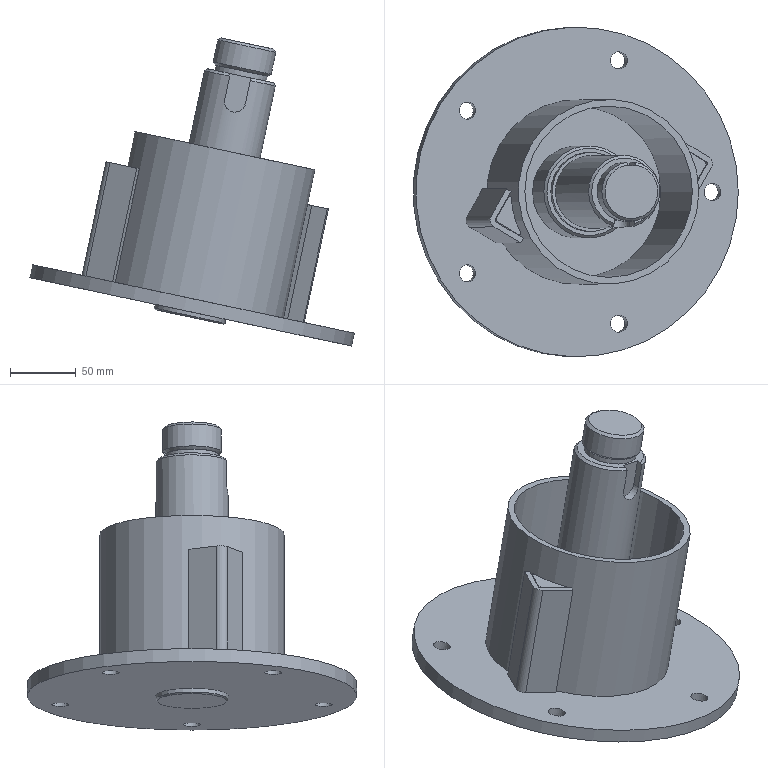Part | STEP file | HL4GZ-1.862.060 (cutter disc mounting flange weldment) | 7 solids | 76 faces | box 246.616 x 250 x 233.706 mm | volume 1291217 mm3 | plane 43 | cylinder 27 | cone 6 | commonest cylinder face diameters 13 x5 2 x4 55 x3 140 x3 4 x2 12 x2